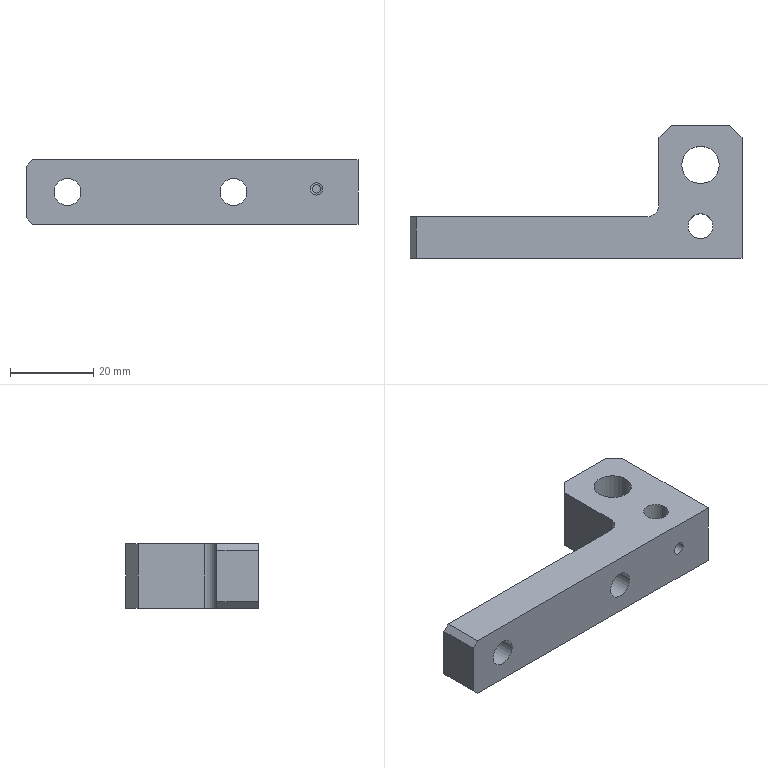NC program | NX | posted with a generic post | part box 80 x 32 x 15.5 mm
Lines 3717 to 3920 of 7013:
(动态粗_COPY , TOOL : D6-18-D6-50-3T-FINISH)
N7396 T06 M6
N7398 G53
N7400 G17 G0 G90 X14.899 Y-0.729 B0. C0. S3500 M3
N7402 G43 Z20. H6
N7404 Z-16.
N7406 G94 G1 X14.924 Z-16.156 F800.
N7408 X14.949 Z-16.218
N7410 X14.974 Z-16.263
N7412 X14.999 Z-16.3
N7414 X15.024 Y-0.728 Z-16.331
N7416 X15.049 Z-16.357
N7418 X15.074 Z-16.38
N7420 X15.099 Z-16.4
N7422 X15.124 Z-16.418
N7424 X15.149 Y-0.727 Z-16.433
N7426 X15.174 Z-16.447
N7428 X15.199 Z-16.458
N7430 X15.224 Z-16.468
N7432 X15.249 Y-0.726 Z-16.477
N7434 X15.274 Z-16.484
N7436 X15.299 Z-16.49
N7438 X15.324 Z-16.494
N7440 X15.349 Z-16.497
N7442 X15.374 Y-0.725 Z-16.499
N7444 X15.399 Z-16.5
N7446 X16.299 Y-0.718
N7448 G3 X16.867 Y0.146 R0.641
N7450 X14.488 Y2.83 R3.165
N7452 G1 X14.195 Y2.9
N7454 X14.
N7456 G2 X15.747 Y2.235 R2.74
N7458 X16.9 Y0.197 R3.187
N7460 G1 Y-0.028
N7462 G3 X15.205 Y2.64 R2.922
N7464 X14.431 Y2.9 R2.405
N7466 G1 X14.213
N7468 G2 X15.783 Y2.306 R2.346
N7470 X16.9 Y0.431 R2.988
N7472 G1 Y0.251
N7474 G3 X16.062 Y2.125 R2.488
N7476 X14.638 Y2.9 R2.746
N7478 G1 X14.458
N7480 G2 X15.807 Y2.385 R2.029
N7482 X16.9 Y0.635 R2.808
N7484 G1 Y0.506
N7486 G3 X16.217 Y2.077 R2.207
N7488 X14.821 Y2.9 R2.429
N7490 G1 X14.671
N7492 G2 X15.918 Y2.395 R1.834
N7494 X16.9 Y0.811 R2.587
N7496 G1 Y0.714
N7498 G3 X16.255 Y2.147 R2.039
N7500 X14.984 Y2.9 R2.173
N7502 G1 X14.857
N7504 G2 X16.023 Y2.404 R1.691
N7506 X16.9 Y0.969 R2.36
N7508 G1 Y0.886
N7510 G3 X16.282 Y2.224 R1.912
N7512 X15.134 Y2.9 R1.959
N7514 G1 X15.02
N7516 G2 X16.128 Y2.409 R1.579
N7518 X16.9 Y1.112 R2.148
N7520 G1 Y1.034
N7522 G3 X16.281 Y2.326 R1.809
N7524 X15.273 Y2.9 R1.754
N7526 G1 X15.168
N7528 G2 X16.248 Y2.393 R1.505
N7530 X16.9 Y1.251 R1.897
N7532 G1 Y1.176
N7534 G3 X16.277 Y2.424 R1.717
N7536 X15.3 Y2.9 R1.39
N7538 G2 X16.339 Y2.396 R1.416
N7540 X16.9 Y1.307 R1.624
N7542 G3 X16.236 Y2.546 R1.644
N7544 X15.415 Y2.9 R1.188
N7546 G2 X16.415 Y2.407 R1.324
N7548 X16.9 Y1.422 R1.474
N7550 G3 X16.207 Y2.644 R1.556
N7552 X15.531 Y2.9 R0.928
N7554 G2 X16.517 Y2.382 R1.264
N7556 X16.9 Y1.537 R1.316
N7558 G3 X16.144 Y2.75 R1.476
N7560 X15.637 Y2.9 R0.775
N7562 G2 X16.609 Y2.356 R1.207
N7564 X16.9 Y1.647 R1.036
N7566 G3 X15.861 Y2.897 R1.346
N7568 G1 X15.736 Y2.9
N7570 G2 X16.692 Y2.323 R1.148
N7572 X16.9 Y1.748 R0.896
N7574 G3 X15.894 Y2.9 R1.202
N7576 G1 X15.834
N7578 G2 X16.761 Y2.296 R1.086
N7580 X16.9 Y1.835 R0.785
N7582 G3 X15.97 Y2.9 R1.095
N7584 G1 X15.91
N7586 G2 X16.842 Y2.214 R1.034
N7588 X16.9 Y1.923 R0.636
N7590 G3 X15.987 Y2.9 R0.976
N7592 G2 X16.9 Y2.003 R0.945
N7594 G3 X16.056 Y2.9 R0.894
N7596 G2 X16.9 Y2.077 R0.866
N7598 G3 X16.119 Y2.9 R0.819
N7600 G2 X16.9 Y2.134 R0.774
N7602 G3 X16.175 Y2.9 R0.732
N7604 G2 X16.9 Y2.188 R0.713
N7606 G3 X16.21 Y2.9 R0.677
N7608 G2 X16.9 Y2.243 R0.66
N7610 G3 X16.249 Y2.9 R0.631
N7612 G2 X16.897 Y2.331 R0.614
N7614 G1 X16.896 Y2.346
N7616 G3 X16.335 Y2.897 R0.6
N7618 X15.723 Y2.502 R0.606
N7620 G1 X15.317 Y1.398
N7622 X15.308 Y1.374 Z-16.499
N7624 X15.3 Y1.351 Z-16.497
N7626 X15.291 Y1.327 Z-16.494
N7628 X15.282 Y1.304 Z-16.49
N7630 X15.274 Y1.28 Z-16.484
N7632 X15.265 Y1.257 Z-16.477
N7634 X15.257 Y1.233 Z-16.468
N7636 X15.248 Y1.21 Z-16.458
N7638 X15.239 Y1.187 Z-16.447
N7640 X15.231 Y1.163 Z-16.433
N7642 X15.222 Y1.14 Z-16.418
N7644 X15.213 Y1.116 Z-16.4
N7646 X15.205 Y1.093 Z-16.38
N7648 X15.196 Y1.069 Z-16.357
N7650 X15.187 Y1.046 Z-16.331
N7652 X15.179 Y1.022 Z-16.3
N7654 X15.17 Y0.999 Z-16.263
N7656 X15.162 Y0.975 Z-16.218
N7658 X15.153 Y0.952 Z-16.156
N7660 X15.144 Y0.928 Z-16.
N7662 G0 Z20.
(PLANAR_MILL_1 , TOOL : D6-18-D6-50-3T-FINISH)
N7664 X25.116 Y-22.368 S3000
N7666 Z-13.3
N7668 G1 Z-16.3
N7670 X20.874 Y-18.125
N7672 X17.874 Y-15.126
N7674 G2 X16.994 Y-13. R3.006
N7676 G1 Y2.994
N7678 X-40.
N7680 G2 X-43.006 Y6. R3.006
N7682 G1 Y16.
N7684 G2 X-40. Y19.006 R3.006
N7686 G1 X40.
N7688 G2 X43.006 Y16. R3.006
N7690 G1 Y-13.
N7692 G2 X42.126 Y-15.126 R3.006
N7694 G1 X39.126 Y-18.126
N7696 G2 X37. Y-19.006 R3.006
N7698 G1 X23.001
N7700 X17.001
N7702 Z-13.3
N7704 G0 Z20.
N7706 X25.119 Y-22.366
N7708 Z-13.3
N7710 G1 Z-16.3
N7712 X20.876 Y-18.123
N7714 X17.877 Y-15.123
N7716 G2 X16.997 Y-13. R3.003
N7718 G1 Y2.997
N7720 X-40.
N7722 G2 X-43.003 Y6. R3.003
N7724 G1 Y16.
N7726 G2 X-40. Y19.003 R3.003
N7728 G1 X40.
N7730 G2 X43.003 Y16. R3.003
N7732 G1 Y-13.
N7734 G2 X42.123 Y-15.123 R3.003
N7736 G1 X39.123 Y-18.123
N7738 G2 X37. Y-19.003 R3.003
N7740 G1 X23.001
N7742 X17.001
N7744 Z-13.3
N7746 G0 Z20.
N7748 X25.121 Y-22.363
N7750 Z-13.3
N7752 G1 Z-16.3
N7754 X20.878 Y-18.121
N7756 X17.879 Y-15.121
N7758 G2 X17. Y-13. R3.
N7760 G1 Y3.
N7762 X-40.
N7764 G2 X-43. Y6. R3.
N7766 G1 Y16.
N7768 G2 X-40. Y19. R3.
N7770 G1 X40.
N7772 G2 X43. Y16. R3.
N7774 G1 Y-13.
N7776 G2 X42.121 Y-15.121 R3.
N7778 G1 X39.121 Y-18.121
N7780 G2 X37. Y-19. R3.
N7782 G1 X23.001
N7784 X17.001
N7786 Z-13.3
N7788 G0 Z20.
N7790 M5